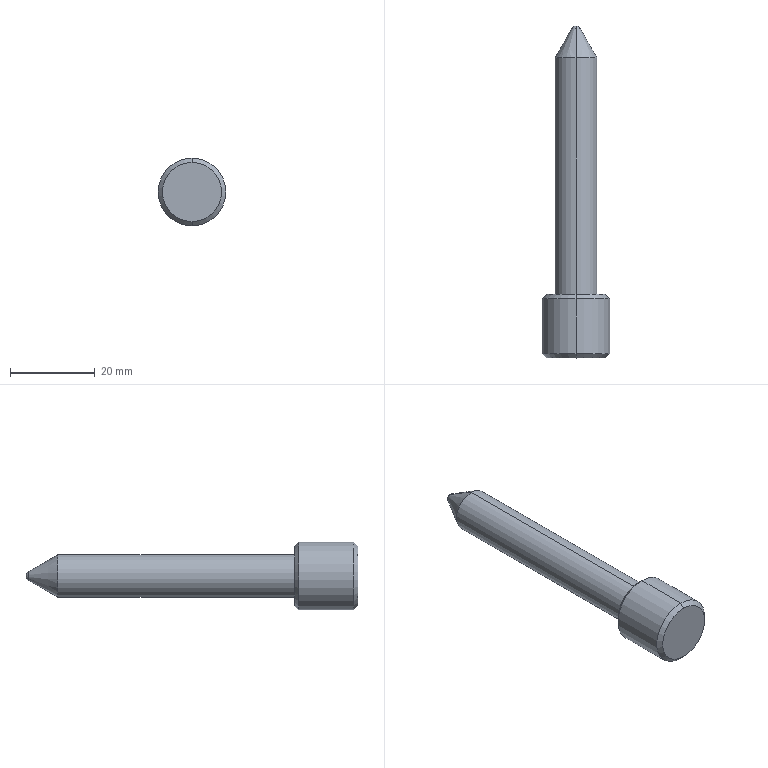Part | SolidWorks | features Chamfer 1, Revolution 1 | 1 solid | 15 faces | box 16 x 78.492 x 16 mm | volume 7592 mm3 | cone 6 | cylinder 4 | plane 3 | torus 2 | commonest cylinder face diameters 10 x2 16 x2
STEP:
#1=CARTESIAN_POINT('',(0.,0.,-7.));
#2=VERTEX_POINT('',#1);
#3=CARTESIAN_POINT('',(0.,0.,7.));
#4=VERTEX_POINT('',#3);
#5=CARTESIAN_POINT('',(0.,0.,0.));
#6=DIRECTION('',(0.,-1.,0.));
#7=DIRECTION('',(0.,0.,1.));
#8=AXIS2_PLACEMENT_3D('',#5,#6,#7);
#9=CIRCLE('',#8,7.);
#10=EDGE_CURVE('',#2,#4,#9,.T.);
#11=ORIENTED_EDGE('',*,*,#10,.F.);
#12=CARTESIAN_POINT('',(0.,1.,-8.));
#13=VERTEX_POINT('',#12);
#14=CARTESIAN_POINT('',(0.,0.,-7.));
#15=DIRECTION('',(0.,0.7071,-0.7071));
#16=VECTOR('',#15,1000.);
#17=LINE('',#14,#16);
#18=EDGE_CURVE('',#2,#13,#17,.T.);
#19=ORIENTED_EDGE('',*,*,#18,.T.);
#20=CARTESIAN_POINT('',(0.,1.,8.));
#21=VERTEX_POINT('',#20);
#22=CARTESIAN_POINT('',(0.,1.,0.));
#23=DIRECTION('',(0.,1.,0.));
#24=DIRECTION('',(0.,0.,1.));
#25=AXIS2_PLACEMENT_3D('',#22,#23,#24);
#26=CIRCLE('',#25,8.);
#27=EDGE_CURVE('',#21,#13,#26,.T.);
#28=ORIENTED_EDGE('',*,*,#27,.F.);
#29=CARTESIAN_POINT('',(0.,0.,7.));
#30=DIRECTION('',(0.,0.7071,0.7071));
#31=VECTOR('',#30,1000.);
#32=LINE('',#29,#31);
#33=EDGE_CURVE('',#4,#21,#32,.T.);
#34=ORIENTED_EDGE('',*,*,#33,.F.);
#35=EDGE_LOOP('',(#11,#19,#28,#34));
#36=FACE_OUTER_BOUND('',#35,.T.);
#37=CARTESIAN_POINT('',(0.,0.,0.));
#38=DIRECTION('',(0.,1.,0.));
#39=DIRECTION('',(0.,0.,1.));
#40=AXIS2_PLACEMENT_3D('',#37,#38,#39);
#41=CONICAL_SURFACE('',#40,7.,0.7854);
#42=ADVANCED_FACE('',(#36),#41,.T.);
#43=CARTESIAN_POINT('',(0.,15.,7.));
#44=VERTEX_POINT('',#43);
#45=CARTESIAN_POINT('',(0.,15.,-7.));
#46=VERTEX_POINT('',#45);
#47=CARTESIAN_POINT('',(0.,15.,0.));
#48=DIRECTION('',(0.,1.,0.));
#49=DIRECTION('',(0.,0.,-1.));
#50=AXIS2_PLACEMENT_3D('',#47,#48,#49);
#51=CIRCLE('',#50,7.);
#52=EDGE_CURVE('',#44,#46,#51,.T.);
#53=ORIENTED_EDGE('',*,*,#52,.F.);
#54=CARTESIAN_POINT('',(0.,14.,8.));
#55=VERTEX_POINT('',#54);
#56=CARTESIAN_POINT('',(0.,14.,8.));
#57=DIRECTION('',(0.,-0.7071,0.7071));
#58=VECTOR('',#57,1000.);
#59=LINE('',#56,#58);
#60=EDGE_CURVE('',#44,#55,#59,.T.);
#61=ORIENTED_EDGE('',*,*,#60,.T.);
#62=CARTESIAN_POINT('',(0.,14.,-8.));
#63=VERTEX_POINT('',#62);
#64=CARTESIAN_POINT('',(0.,14.,0.));
#65=DIRECTION('',(0.,-1.,0.));
#66=DIRECTION('',(0.,0.,-1.));
#67=AXIS2_PLACEMENT_3D('',#64,#65,#66);
#68=CIRCLE('',#67,8.);
#69=EDGE_CURVE('',#63,#55,#68,.T.);
#70=ORIENTED_EDGE('',*,*,#69,.F.);
#71=CARTESIAN_POINT('',(0.,14.,-8.));
#72=DIRECTION('',(0.,-0.7071,-0.7071));
#73=VECTOR('',#72,1000.);
#74=LINE('',#71,#73);
#75=EDGE_CURVE('',#46,#63,#74,.T.);
#76=ORIENTED_EDGE('',*,*,#75,.F.);
#77=EDGE_LOOP('',(#53,#61,#70,#76));
#78=FACE_OUTER_BOUND('',#77,.T.);
#79=CARTESIAN_POINT('',(0.,14.,0.));
#80=DIRECTION('',(0.,-1.,0.));
#81=DIRECTION('',(0.,0.,-1.));
#82=AXIS2_PLACEMENT_3D('',#79,#80,#81);
#83=CONICAL_SURFACE('',#82,8.,0.7854);
#84=ADVANCED_FACE('',(#78),#83,.T.);
#85=ORIENTED_EDGE('',*,*,#69,.T.);
#86=CARTESIAN_POINT('',(0.,0.,8.));
#87=DIRECTION('',(0.,-1.,0.));
#88=VECTOR('',#87,1000.);
#89=LINE('',#86,#88);
#90=EDGE_CURVE('',#55,#21,#89,.T.);
#91=ORIENTED_EDGE('',*,*,#90,.T.);
#92=ORIENTED_EDGE('',*,*,#27,.T.);
#93=CARTESIAN_POINT('',(0.,0.,-8.));
#94=DIRECTION('',(0.,-1.,0.));
#95=VECTOR('',#94,1000.);
#96=LINE('',#93,#95);
#97=EDGE_CURVE('',#63,#13,#96,.T.);
#98=ORIENTED_EDGE('',*,*,#97,.F.);
#99=EDGE_LOOP('',(#85,#91,#92,#98));
#100=FACE_OUTER_BOUND('',#99,.T.);
#101=CARTESIAN_POINT('',(0.,0.,0.));
#102=DIRECTION('',(0.,-1.,0.));
#103=DIRECTION('',(0.,0.,-1.));
#104=AXIS2_PLACEMENT_3D('',#101,#102,#103);
#105=CYLINDRICAL_SURFACE('',#104,8.);
#106=ADVANCED_FACE('',(#100),#105,.T.);
#107=CARTESIAN_POINT('',(0.,71.,-5.));
#108=VERTEX_POINT('',#107);
#109=CARTESIAN_POINT('',(0.,71.,5.));
#110=VERTEX_POINT('',#109);
#111=CARTESIAN_POINT('',(0.,71.,0.));
#112=DIRECTION('',(0.,-1.,0.));
#113=DIRECTION('',(0.,0.,-1.));
#114=AXIS2_PLACEMENT_3D('',#111,#112,#113);
#115=CIRCLE('',#114,5.);
#116=EDGE_CURVE('',#108,#110,#115,.T.);
#117=ORIENTED_EDGE('',*,*,#116,.T.);
#118=CARTESIAN_POINT('',(0.,15.,5.));
#119=VERTEX_POINT('',#118);
#120=CARTESIAN_POINT('',(0.,0.,5.));
#121=DIRECTION('',(0.,-1.,0.));
#122=VECTOR('',#121,1000.);
#123=LINE('',#120,#122);
#124=EDGE_CURVE('',#110,#119,#123,.T.);
#125=ORIENTED_EDGE('',*,*,#124,.T.);
#126=CARTESIAN_POINT('',(0.,15.,-5.));
#127=VERTEX_POINT('',#126);
#128=CARTESIAN_POINT('',(0.,15.,0.));
#129=DIRECTION('',(0.,-1.,0.));
#130=DIRECTION('',(0.,0.,-1.));
#131=AXIS2_PLACEMENT_3D('',#128,#129,#130);
#132=CIRCLE('',#131,5.);
#133=EDGE_CURVE('',#127,#119,#132,.T.);
#134=ORIENTED_EDGE('',*,*,#133,.F.);
#135=CARTESIAN_POINT('',(0.,0.,-5.));
#136=DIRECTION('',(0.,-1.,0.));
#137=VECTOR('',#136,1000.);
#138=LINE('',#135,#137);
#139=EDGE_CURVE('',#108,#127,#138,.T.);
#140=ORIENTED_EDGE('',*,*,#139,.F.);
#141=EDGE_LOOP('',(#117,#125,#134,#140));
#142=FACE_OUTER_BOUND('',#141,.T.);
#143=CARTESIAN_POINT('',(0.,0.,0.));
#144=DIRECTION('',(0.,-1.,0.));
#145=DIRECTION('',(0.,0.,-1.));
#146=AXIS2_PLACEMENT_3D('',#143,#144,#145);
#147=CYLINDRICAL_SURFACE('',#146,5.);
#148=ADVANCED_FACE('',(#142),#147,.T.);
#149=CARTESIAN_POINT('',(0.,77.992,-0.9634));
#150=VERTEX_POINT('',#149);
#151=CARTESIAN_POINT('',(0.,77.992,0.9634));
#152=VERTEX_POINT('',#151);
#153=CARTESIAN_POINT('',(0.,77.992,0.));
#154=DIRECTION('',(0.,-1.,0.));
#155=DIRECTION('',(0.,0.,-1.));
#156=AXIS2_PLACEMENT_3D('',#153,#154,#155);
#157=CIRCLE('',#156,0.9634);
#158=EDGE_CURVE('',#150,#152,#157,.T.);
#159=ORIENTED_EDGE('',*,*,#158,.T.);
#160=CARTESIAN_POINT('',(0.,77.992,0.9634));
#161=DIRECTION('',(0.,-0.866,0.5));
#162=VECTOR('',#161,1000.);
#163=LINE('',#160,#162);
#164=EDGE_CURVE('',#152,#110,#163,.T.);
#165=ORIENTED_EDGE('',*,*,#164,.T.);
#166=ORIENTED_EDGE('',*,*,#116,.F.);
#167=CARTESIAN_POINT('',(0.,77.992,-0.9634));
#168=DIRECTION('',(0.,-0.866,-0.5));
#169=VECTOR('',#168,1000.);
#170=LINE('',#167,#169);
#171=EDGE_CURVE('',#150,#108,#170,.T.);
#172=ORIENTED_EDGE('',*,*,#171,.F.);
#173=EDGE_LOOP('',(#159,#165,#166,#172));
#174=FACE_OUTER_BOUND('',#173,.T.);
#175=CARTESIAN_POINT('',(0.,77.992,0.));
#176=DIRECTION('',(0.,-1.,0.));
#177=DIRECTION('',(0.,0.,-1.));
#178=AXIS2_PLACEMENT_3D('',#175,#176,#177);
#179=CONICAL_SURFACE('',#178,0.9634,0.5236);
#180=ADVANCED_FACE('',(#174),#179,.T.);
#181=CARTESIAN_POINT('',(0.,78.492,-0.09737));
#182=VERTEX_POINT('',#181);
#183=CARTESIAN_POINT('',(0.,78.492,0.09737));
#184=VERTEX_POINT('',#183);
#185=CARTESIAN_POINT('',(0.,78.492,0.));
#186=DIRECTION('',(0.,-1.,0.));
#187=DIRECTION('',(0.,0.,-1.));
#188=AXIS2_PLACEMENT_3D('',#185,#186,#187);
#189=CIRCLE('',#188,0.09737);
#190=EDGE_CURVE('',#182,#184,#189,.T.);
#191=ORIENTED_EDGE('',*,*,#190,.T.);
#192=CARTESIAN_POINT('',(0.,77.492,0.09737));
#193=DIRECTION('',(1.,0.,0.));
#194=DIRECTION('',(0.,0.,-1.));
#195=AXIS2_PLACEMENT_3D('',#192,#193,#194);
#196=CIRCLE('',#195,1.);
#197=EDGE_CURVE('',#184,#152,#196,.T.);
#198=ORIENTED_EDGE('',*,*,#197,.T.);
#199=ORIENTED_EDGE('',*,*,#158,.F.);
#200=CARTESIAN_POINT('',(0.,77.492,-0.09737));
#201=DIRECTION('',(-1.,0.,0.));
#202=DIRECTION('',(0.,0.,1.));
#203=AXIS2_PLACEMENT_3D('',#200,#201,#202);
#204=CIRCLE('',#203,1.);
#205=EDGE_CURVE('',#182,#150,#204,.T.);
#206=ORIENTED_EDGE('',*,*,#205,.F.);
#207=EDGE_LOOP('',(#191,#198,#199,#206));
#208=FACE_OUTER_BOUND('',#207,.T.);
#209=CARTESIAN_POINT('',(0.,77.492,0.));
#210=DIRECTION('',(0.,-1.,0.));
#211=DIRECTION('',(0.,0.,-1.));
#212=AXIS2_PLACEMENT_3D('',#209,#210,#211);
#213=TOROIDAL_SURFACE('',#212,0.09737,1.);
#214=ADVANCED_FACE('',(#208),#213,.T.);
#215=ORIENTED_EDGE('',*,*,#190,.F.);
#216=CARTESIAN_POINT('',(0.,78.492,0.));
#217=DIRECTION('',(0.,-1.,0.));
#218=DIRECTION('',(0.,0.,-1.));
#219=AXIS2_PLACEMENT_3D('',#216,#217,#218);
#220=CIRCLE('',#219,0.09737);
#221=EDGE_CURVE('',#184,#182,#220,.T.);
#222=ORIENTED_EDGE('',*,*,#221,.F.);
#223=EDGE_LOOP('',(#215,#222));
#224=FACE_OUTER_BOUND('',#223,.T.);
#225=CARTESIAN_POINT('',(-0.09737,78.492,0.));
#226=DIRECTION('',(0.,-1.,0.));
#227=DIRECTION('',(0.,0.,-1.));
#228=AXIS2_PLACEMENT_3D('',#225,#226,#227);
#229=PLANE('',#228);
#230=ADVANCED_FACE('',(#224),#229,.F.);
#231=ORIENTED_EDGE('',*,*,#197,.F.);
#232=ORIENTED_EDGE('',*,*,#221,.T.);
#233=ORIENTED_EDGE('',*,*,#205,.T.);
#234=CARTESIAN_POINT('',(0.,77.992,0.));
#235=DIRECTION('',(0.,-1.,0.));
#236=DIRECTION('',(0.,0.,-1.));
#237=AXIS2_PLACEMENT_3D('',#234,#235,#236);
#238=CIRCLE('',#237,0.9634);
#239=EDGE_CURVE('',#152,#150,#238,.T.);
#240=ORIENTED_EDGE('',*,*,#239,.F.);
#241=EDGE_LOOP('',(#231,#232,#233,#240));
#242=FACE_OUTER_BOUND('',#241,.T.);
#243=CARTESIAN_POINT('',(0.,77.492,0.));
#244=DIRECTION('',(0.,-1.,0.));
#245=DIRECTION('',(0.,0.,-1.));
#246=AXIS2_PLACEMENT_3D('',#243,#244,#245);
#247=TOROIDAL_SURFACE('',#246,0.09737,1.);
#248=ADVANCED_FACE('',(#242),#247,.T.);
#249=ORIENTED_EDGE('',*,*,#164,.F.);
#250=ORIENTED_EDGE('',*,*,#239,.T.);
#251=ORIENTED_EDGE('',*,*,#171,.T.);
#252=CARTESIAN_POINT('',(0.,71.,0.));
#253=DIRECTION('',(0.,-1.,0.));
#254=DIRECTION('',(0.,0.,-1.));
#255=AXIS2_PLACEMENT_3D('',#252,#253,#254);
#256=CIRCLE('',#255,5.);
#257=EDGE_CURVE('',#110,#108,#256,.T.);
#258=ORIENTED_EDGE('',*,*,#257,.F.);
#259=EDGE_LOOP('',(#249,#250,#251,#258));
#260=FACE_OUTER_BOUND('',#259,.T.);
#261=CARTESIAN_POINT('',(0.,77.992,0.));
#262=DIRECTION('',(0.,-1.,0.));
#263=DIRECTION('',(0.,0.,-1.));
#264=AXIS2_PLACEMENT_3D('',#261,#262,#263);
#265=CONICAL_SURFACE('',#264,0.9634,0.5236);
#266=ADVANCED_FACE('',(#260),#265,.T.);
#267=ORIENTED_EDGE('',*,*,#124,.F.);
#268=ORIENTED_EDGE('',*,*,#257,.T.);
#269=ORIENTED_EDGE('',*,*,#139,.T.);
#270=CARTESIAN_POINT('',(0.,15.,0.));
#271=DIRECTION('',(0.,-1.,0.));
#272=DIRECTION('',(0.,0.,-1.));
#273=AXIS2_PLACEMENT_3D('',#270,#271,#272);
#274=CIRCLE('',#273,5.);
#275=EDGE_CURVE('',#119,#127,#274,.T.);
#276=ORIENTED_EDGE('',*,*,#275,.F.);
#277=EDGE_LOOP('',(#267,#268,#269,#276));
#278=FACE_OUTER_BOUND('',#277,.T.);
#279=CARTESIAN_POINT('',(0.,0.,0.));
#280=DIRECTION('',(0.,-1.,0.));
#281=DIRECTION('',(0.,0.,-1.));
#282=AXIS2_PLACEMENT_3D('',#279,#280,#281);
#283=CYLINDRICAL_SURFACE('',#282,5.);
#284=ADVANCED_FACE('',(#278),#283,.T.);
#285=CARTESIAN_POINT('',(0.,15.,0.));
#286=DIRECTION('',(0.,1.,0.));
#287=DIRECTION('',(0.,0.,-1.));
#288=AXIS2_PLACEMENT_3D('',#285,#286,#287);
#289=CIRCLE('',#288,7.);
#290=EDGE_CURVE('',#46,#44,#289,.T.);
#291=ORIENTED_EDGE('',*,*,#290,.T.);
#292=ORIENTED_EDGE('',*,*,#52,.T.);
#293=EDGE_LOOP('',(#291,#292));
#294=FACE_OUTER_BOUND('',#293,.T.);
#295=ORIENTED_EDGE('',*,*,#133,.T.);
#296=ORIENTED_EDGE('',*,*,#275,.T.);
#297=EDGE_LOOP('',(#295,#296));
#298=FACE_BOUND('',#297,.T.);
#299=CARTESIAN_POINT('',(-5.,15.,0.));
#300=DIRECTION('',(0.,-1.,0.));
#301=DIRECTION('',(0.,0.,-1.));
#302=AXIS2_PLACEMENT_3D('',#299,#300,#301);
#303=PLANE('',#302);
#304=ADVANCED_FACE('',(#294,#298),#303,.F.);
#305=ORIENTED_EDGE('',*,*,#90,.F.);
#306=CARTESIAN_POINT('',(0.,14.,0.));
#307=DIRECTION('',(0.,-1.,0.));
#308=DIRECTION('',(0.,0.,-1.));
#309=AXIS2_PLACEMENT_3D('',#306,#307,#308);
#310=CIRCLE('',#309,8.);
#311=EDGE_CURVE('',#55,#63,#310,.T.);
#312=ORIENTED_EDGE('',*,*,#311,.T.);
#313=ORIENTED_EDGE('',*,*,#97,.T.);
#314=CARTESIAN_POINT('',(0.,1.,0.));
#315=DIRECTION('',(0.,1.,0.));
#316=DIRECTION('',(0.,0.,1.));
#317=AXIS2_PLACEMENT_3D('',#314,#315,#316);
#318=CIRCLE('',#317,8.);
#319=EDGE_CURVE('',#13,#21,#318,.T.);
#320=ORIENTED_EDGE('',*,*,#319,.T.);
#321=EDGE_LOOP('',(#305,#312,#313,#320));
#322=FACE_OUTER_BOUND('',#321,.T.);
#323=CARTESIAN_POINT('',(0.,0.,0.));
#324=DIRECTION('',(0.,-1.,0.));
#325=DIRECTION('',(0.,0.,-1.));
#326=AXIS2_PLACEMENT_3D('',#323,#324,#325);
#327=CYLINDRICAL_SURFACE('',#326,8.);
#328=ADVANCED_FACE('',(#322),#327,.T.);
#329=CARTESIAN_POINT('',(0.,0.,0.));
#330=DIRECTION('',(0.,-1.,0.));
#331=DIRECTION('',(0.,0.,1.));
#332=AXIS2_PLACEMENT_3D('',#329,#330,#331);
#333=CIRCLE('',#332,7.);
#334=EDGE_CURVE('',#4,#2,#333,.T.);
#335=ORIENTED_EDGE('',*,*,#334,.T.);
#336=ORIENTED_EDGE('',*,*,#10,.T.);
#337=EDGE_LOOP('',(#335,#336));
#338=FACE_OUTER_BOUND('',#337,.T.);
#339=CARTESIAN_POINT('',(-8.,0.,0.));
#340=DIRECTION('',(0.,1.,0.));
#341=DIRECTION('',(0.,0.,1.));
#342=AXIS2_PLACEMENT_3D('',#339,#340,#341);
#343=PLANE('',#342);
#344=ADVANCED_FACE('',(#338),#343,.F.);
#345=ORIENTED_EDGE('',*,*,#60,.F.);
#346=ORIENTED_EDGE('',*,*,#290,.F.);
#347=ORIENTED_EDGE('',*,*,#75,.T.);
#348=ORIENTED_EDGE('',*,*,#311,.F.);
#349=EDGE_LOOP('',(#345,#346,#347,#348));
#350=FACE_OUTER_BOUND('',#349,.T.);
#351=CARTESIAN_POINT('',(0.,14.,0.));
#352=DIRECTION('',(0.,-1.,0.));
#353=DIRECTION('',(0.,0.,-1.));
#354=AXIS2_PLACEMENT_3D('',#351,#352,#353);
#355=CONICAL_SURFACE('',#354,8.,0.7854);
#356=ADVANCED_FACE('',(#350),#355,.T.);
#357=ORIENTED_EDGE('',*,*,#18,.F.);
#358=ORIENTED_EDGE('',*,*,#334,.F.);
#359=ORIENTED_EDGE('',*,*,#33,.T.);
#360=ORIENTED_EDGE('',*,*,#319,.F.);
#361=EDGE_LOOP('',(#357,#358,#359,#360));
#362=FACE_OUTER_BOUND('',#361,.T.);
#363=CARTESIAN_POINT('',(0.,0.,0.));
#364=DIRECTION('',(0.,1.,0.));
#365=DIRECTION('',(0.,0.,1.));
#366=AXIS2_PLACEMENT_3D('',#363,#364,#365);
#367=CONICAL_SURFACE('',#366,7.,0.7854);
#368=ADVANCED_FACE('',(#362),#367,.T.);
#369=CLOSED_SHELL('',(#42,#84,#106,#148,#180,#214,#230,#248,#266,#284,#304,#328,#344,#356,#368));
#370=MANIFOLD_SOLID_BREP('',#369);
#371=CARTESIAN_POINT('',(0.,0.,0.));
#372=DIRECTION('',(0.,0.,1.));
#373=DIRECTION('',(1.,0.,0.));
#374=AXIS2_PLACEMENT_3D('',#371,#372,#373);
#375=(LENGTH_UNIT()NAMED_UNIT(*)SI_UNIT(.MILLI.,.METRE.));
#376=UNCERTAINTY_MEASURE_WITH_UNIT(LENGTH_MEASURE(0.00001),#375,'','');
#377=(NAMED_UNIT(*)PLANE_ANGLE_UNIT()SI_UNIT($,.RADIAN.));
#378=(NAMED_UNIT(*)SI_UNIT($,.STERADIAN.)SOLID_ANGLE_UNIT());
#379=(GEOMETRIC_REPRESENTATION_CONTEXT(3)GLOBAL_UNCERTAINTY_ASSIGNED_CONTEXT((#376))GLOBAL_UNIT_ASSIGNED_CONTEXT((#375,#377,#378))REPRESENTATION_CONTEXT('',''));
#380=ADVANCED_BREP_SHAPE_REPRESENTATION('',(#370,#374),#379);